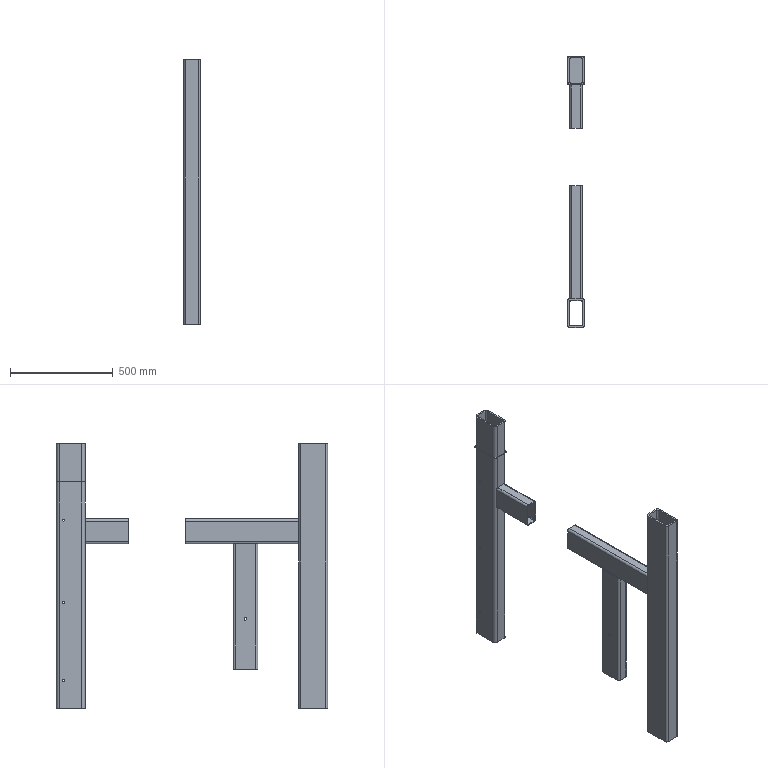Part | STEP file | 1 exported frame w
hy_stp | 7 solids | 122 faces | box 80 x 1320 x 1285 mm | volume 10409301 mm3 | plane 66 | cylinder 56 | commonest cylinder face diameters 10 x18 20 x16 16 x12 32 x8 14 x2